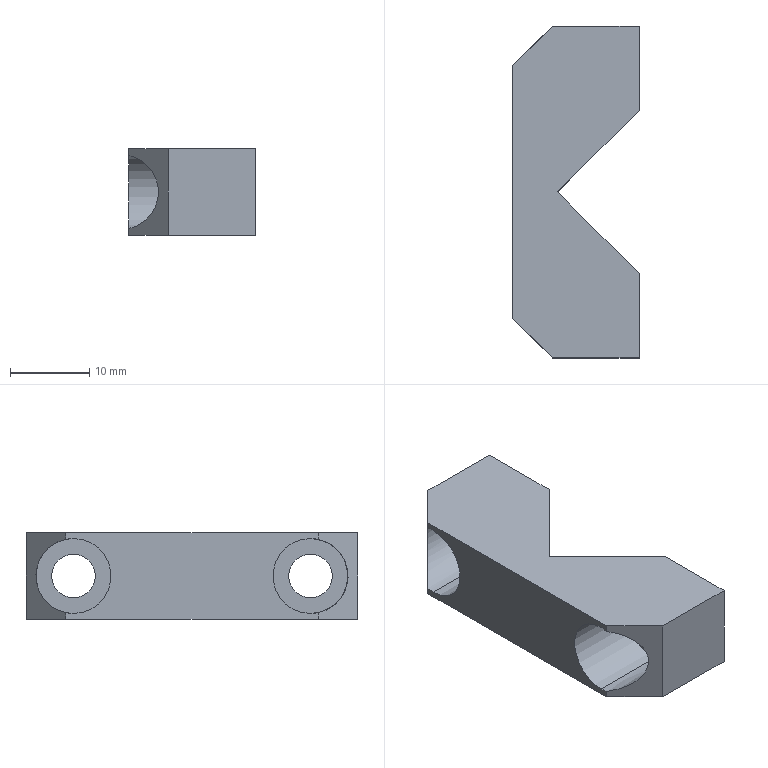Part | STEP file | CLAMP.ARM.2.stp | 1 solid | 21 faces | box 16 x 42 x 11 mm | volume 4382 mm3 | spline 16 | cylinder 4 | plane 1 | commonest cylinder face diameters 5.5 x2 9.5 x2